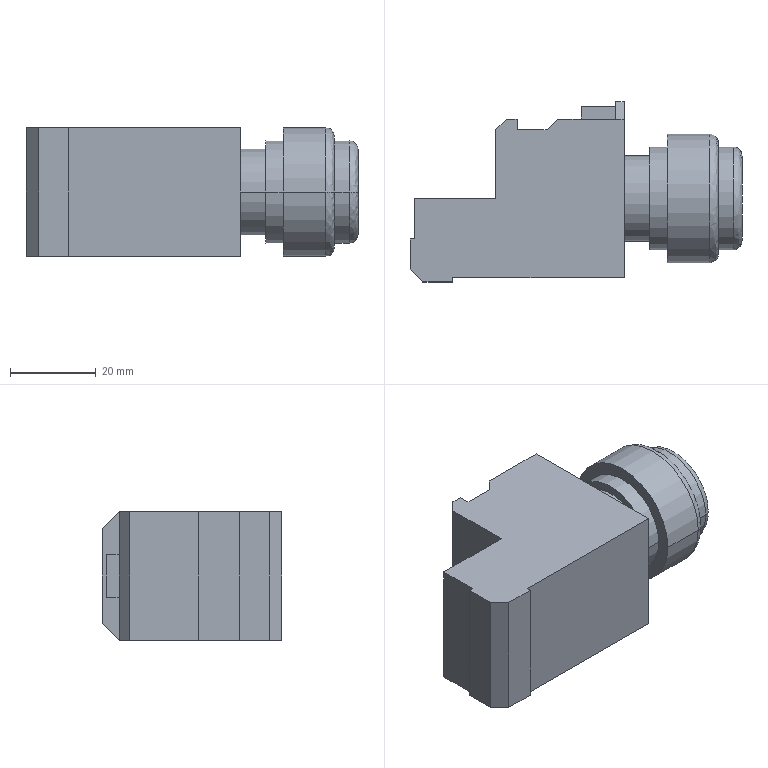Part | STEP file | Start button AR22EOL-10E3G_Fuji1_default | 1 solid | 42 faces | box 77.5 x 42 x 30 mm | volume 58541 mm3 | plane 30 | cylinder 8 | spline 4 | commonest cylinder face diameters 24 x4 20 x2 30 x2